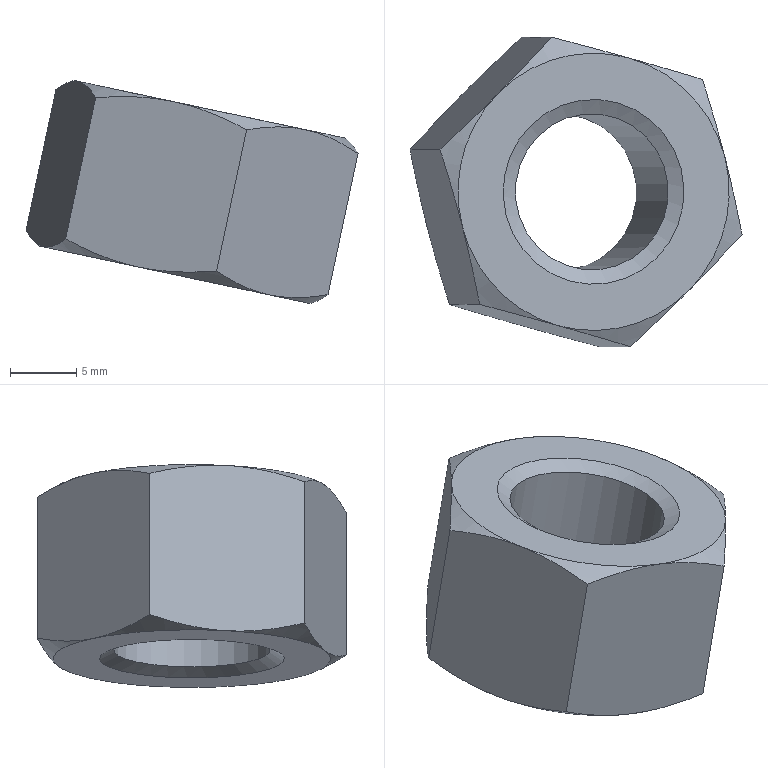Part | STEP file | 8902-M14 nut | 1 solid | 23 faces | box 25.147 x 23.458 x 16.886 mm | volume 3434 mm3 | cone 14 | plane 8 | cylinder 1 | commonest cylinder face diameters 11.835 x1